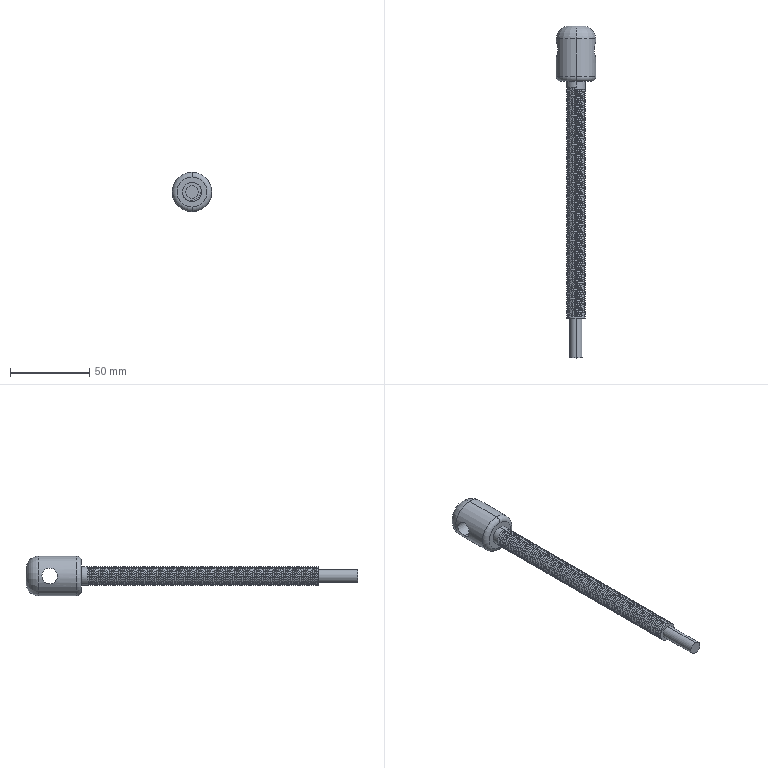Part | SolidWorks | features ICE 3, Fillet 2, Extrusion 1, SweepThread 1 | 1 solid | 227 faces | box 25 x 210 x 25 mm | volume 30147 mm3 | cylinder 214 | plane 6 | torus 4 | spline 3 | commonest cylinder face diameters 12 x208 8 x2 10 x2 25 x2